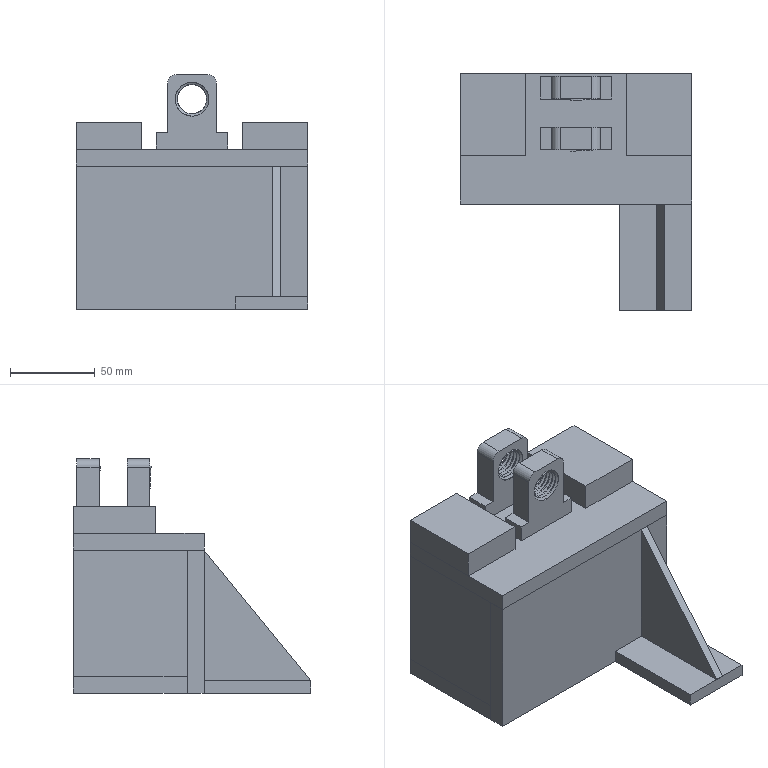Part | SolidWorks | features BaseBody 6, ICE 3, MoveCopyBody 2, SweepThread 2 | 11 solids | 117 faces | box 137.013 x 140.341 x 138.543 mm | volume 535591 mm3 | plane 77 | cylinder 32 | spline 8 | commonest cylinder face diameters 20 x24 10 x8